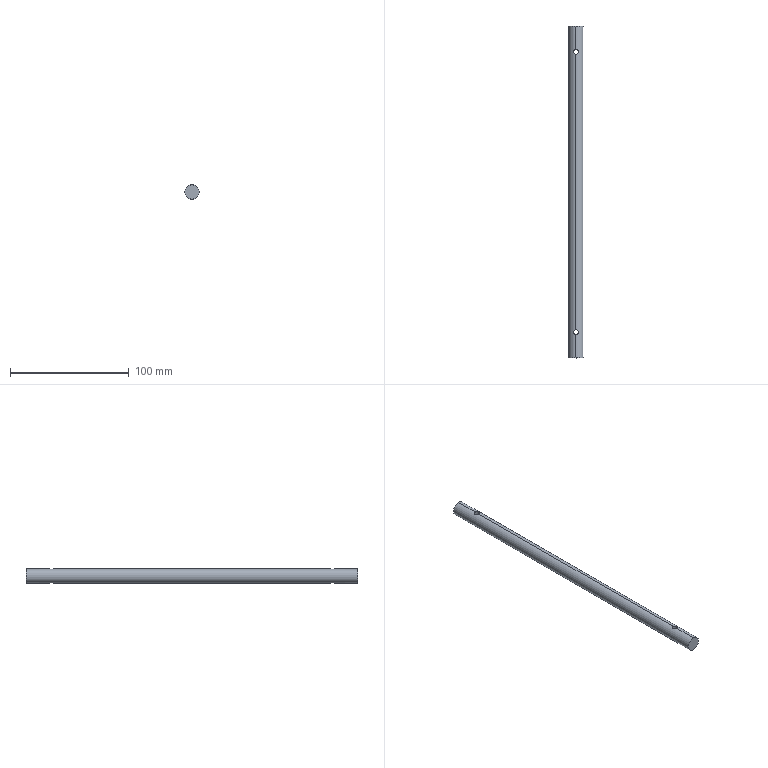Part | SolidWorks | features Extrusion 1, ICE 1, MirrorPattern 1 | 1 solid | 8 faces | box 12 x 280 x 12 mm | volume 31370 mm3 | cylinder 6 | plane 2 | commonest cylinder face diameters 4 x4 12 x2
STEP:
#1=CARTESIAN_POINT('',(0.,116.208,-6.));
#2=VERTEX_POINT('',#1);
#3=CARTESIAN_POINT('',(-2.,118.208,-5.657));
#4=VERTEX_POINT('',#3);
#5=CARTESIAN_POINT('',(0.,116.208,-6.));
#6=CARTESIAN_POINT('',(-0.2623,116.208,-6.));
#7=CARTESIAN_POINT('',(-0.5271,116.261,-5.982));
#8=CARTESIAN_POINT('',(-0.889,116.412,-5.935));
#9=CARTESIAN_POINT('',(-1.006,116.475,-5.916));
#10=CARTESIAN_POINT('',(-1.222,116.619,-5.875));
#11=CARTESIAN_POINT('',(-1.322,116.702,-5.853));
#12=CARTESIAN_POINT('',(-1.599,116.979,-5.786));
#13=CARTESIAN_POINT('',(-1.745,117.197,-5.741));
#14=CARTESIAN_POINT('',(-1.897,117.561,-5.692));
#15=CARTESIAN_POINT('',(-1.935,117.686,-5.679));
#16=CARTESIAN_POINT('',(-1.987,117.943,-5.662));
#17=CARTESIAN_POINT('',(-2.,118.076,-5.657));
#18=CARTESIAN_POINT('',(-2.,118.208,-5.657));
#19=B_SPLINE_CURVE_WITH_KNOTS('',3,(#5,#6,#7,#8,#9,#10,#11,#12,#13,#14,#15,#16,#17,#18),.UNSPECIFIED.,.F.,.F.,(4,2,2,2,2,2,4),(0.006298,0.007085,0.007479,0.007872,0.008659,0.009053,0.009446),.UNSPECIFIED.);
#20=EDGE_CURVE('',#2,#4,#19,.T.);
#21=ORIENTED_EDGE('',*,*,#20,.T.);
#22=CARTESIAN_POINT('',(-2.,118.208,5.657));
#23=VERTEX_POINT('',#22);
#24=CARTESIAN_POINT('',(-2.,118.208,-49.));
#25=DIRECTION('',(0.,0.,1.));
#26=VECTOR('',#25,1000.);
#27=LINE('',#24,#26);
#28=EDGE_CURVE('',#4,#23,#27,.T.);
#29=ORIENTED_EDGE('',*,*,#28,.T.);
#30=CARTESIAN_POINT('',(0.,116.208,6.));
#31=VERTEX_POINT('',#30);
#32=CARTESIAN_POINT('',(-2.,118.208,5.657));
#33=CARTESIAN_POINT('',(-2.,117.946,5.657));
#34=CARTESIAN_POINT('',(-1.947,117.681,5.676));
#35=CARTESIAN_POINT('',(-1.796,117.319,5.725));
#36=CARTESIAN_POINT('',(-1.734,117.202,5.745));
#37=CARTESIAN_POINT('',(-1.589,116.987,5.786));
#38=CARTESIAN_POINT('',(-1.507,116.886,5.809));
#39=CARTESIAN_POINT('',(-1.23,116.609,5.876));
#40=CARTESIAN_POINT('',(-1.012,116.463,5.919));
#41=CARTESIAN_POINT('',(-0.6469,116.311,5.966));
#42=CARTESIAN_POINT('',(-0.5219,116.273,5.979));
#43=CARTESIAN_POINT('',(-0.2652,116.221,5.996));
#44=CARTESIAN_POINT('',(-0.1318,116.208,6.));
#45=CARTESIAN_POINT('',(0.,116.208,6.));
#46=B_SPLINE_CURVE_WITH_KNOTS('',3,(#32,#33,#34,#35,#36,#37,#38,#39,#40,#41,#42,#43,#44,#45),.UNSPECIFIED.,.F.,.F.,(4,2,2,2,2,2,4),(0.006298,0.007085,0.007479,0.007872,0.008659,0.009053,0.009446),.UNSPECIFIED.);
#47=EDGE_CURVE('',#23,#31,#46,.T.);
#48=ORIENTED_EDGE('',*,*,#47,.T.);
#49=CARTESIAN_POINT('',(2.,118.208,5.657));
#50=VERTEX_POINT('',#49);
#51=CARTESIAN_POINT('',(0.,116.208,6.));
#52=CARTESIAN_POINT('',(0.1318,116.208,6.));
#53=CARTESIAN_POINT('',(0.2623,116.221,5.996));
#54=CARTESIAN_POINT('',(0.5209,116.273,5.979));
#55=CARTESIAN_POINT('',(0.6482,116.312,5.966));
#56=CARTESIAN_POINT('',(1.01,116.462,5.919));
#57=CARTESIAN_POINT('',(1.231,116.611,5.875));
#58=CARTESIAN_POINT('',(1.506,116.886,5.809));
#59=CARTESIAN_POINT('',(1.59,116.988,5.786));
#60=CARTESIAN_POINT('',(1.734,117.204,5.744));
#61=CARTESIAN_POINT('',(1.796,117.318,5.725));
#62=CARTESIAN_POINT('',(1.897,117.56,5.693));
#63=CARTESIAN_POINT('',(1.935,117.687,5.679));
#64=CARTESIAN_POINT('',(1.987,117.944,5.662));
#65=CARTESIAN_POINT('',(2.,118.075,5.657));
#66=CARTESIAN_POINT('',(2.,118.208,5.657));
#67=B_SPLINE_CURVE_WITH_KNOTS('',3,(#51,#52,#53,#54,#55,#56,#57,#58,#59,#60,#61,#62,#63,#64,#65,#66),.UNSPECIFIED.,.F.,.F.,(4,2,2,2,2,2,2,4),(0.009446,0.00984,0.01023,0.01102,0.01141,0.01181,0.0122,0.01259),.UNSPECIFIED.);
#68=EDGE_CURVE('',#31,#50,#67,.T.);
#69=ORIENTED_EDGE('',*,*,#68,.T.);
#70=CARTESIAN_POINT('',(2.,118.208,-5.657));
#71=VERTEX_POINT('',#70);
#72=CARTESIAN_POINT('',(2.,118.208,-49.));
#73=DIRECTION('',(0.,0.,1.));
#74=VECTOR('',#73,1000.);
#75=LINE('',#72,#74);
#76=EDGE_CURVE('',#71,#50,#75,.T.);
#77=ORIENTED_EDGE('',*,*,#76,.F.);
#78=CARTESIAN_POINT('',(2.,118.208,-5.657));
#79=CARTESIAN_POINT('',(2.,118.077,-5.657));
#80=CARTESIAN_POINT('',(1.987,117.943,-5.662));
#81=CARTESIAN_POINT('',(1.935,117.686,-5.679));
#82=CARTESIAN_POINT('',(1.897,117.561,-5.693));
#83=CARTESIAN_POINT('',(1.796,117.317,-5.725));
#84=CARTESIAN_POINT('',(1.734,117.202,-5.745));
#85=CARTESIAN_POINT('',(1.589,116.987,-5.786));
#86=CARTESIAN_POINT('',(1.505,116.885,-5.809));
#87=CARTESIAN_POINT('',(1.321,116.701,-5.853));
#88=CARTESIAN_POINT('',(1.221,116.619,-5.875));
#89=CARTESIAN_POINT('',(1.005,116.474,-5.916));
#90=CARTESIAN_POINT('',(0.8882,116.411,-5.935));
#91=CARTESIAN_POINT('',(0.6474,116.311,-5.966));
#92=CARTESIAN_POINT('',(0.5226,116.273,-5.979));
#93=CARTESIAN_POINT('',(0.2637,116.221,-5.996));
#94=CARTESIAN_POINT('',(0.1311,116.208,-6.));
#95=CARTESIAN_POINT('',(0.,116.208,-6.));
#96=B_SPLINE_CURVE_WITH_KNOTS('',3,(#78,#79,#80,#81,#82,#83,#84,#85,#86,#87,#88,#89,#90,#91,#92,#93,#94,#95),.UNSPECIFIED.,.F.,.F.,(4,2,2,2,2,2,2,2,4),(0.00315,0.003544,0.003937,0.004331,0.004724,0.005118,0.005511,0.005905,0.006298),.UNSPECIFIED.);
#97=EDGE_CURVE('',#71,#2,#96,.T.);
#98=ORIENTED_EDGE('',*,*,#97,.T.);
#99=EDGE_LOOP('',(#21,#29,#48,#69,#77,#98));
#100=FACE_OUTER_BOUND('',#99,.T.);
#101=CARTESIAN_POINT('',(0.,118.208,-49.));
#102=DIRECTION('',(0.,0.,1.));
#103=DIRECTION('',(1.,0.,0.));
#104=AXIS2_PLACEMENT_3D('',#101,#102,#103);
#105=CYLINDRICAL_SURFACE('',#104,2.);
#106=ADVANCED_FACE('',(#100),#105,.F.);
#107=CARTESIAN_POINT('',(-2.,-118.208,-5.657));
#108=VERTEX_POINT('',#107);
#109=CARTESIAN_POINT('',(0.,-120.208,-6.));
#110=VERTEX_POINT('',#109);
#111=CARTESIAN_POINT('',(-2.,-118.208,-5.657));
#112=CARTESIAN_POINT('',(-2.,-118.34,-5.657));
#113=CARTESIAN_POINT('',(-1.987,-118.473,-5.662));
#114=CARTESIAN_POINT('',(-1.935,-118.73,-5.679));
#115=CARTESIAN_POINT('',(-1.897,-118.855,-5.693));
#116=CARTESIAN_POINT('',(-1.796,-119.099,-5.725));
#117=CARTESIAN_POINT('',(-1.734,-119.214,-5.745));
#118=CARTESIAN_POINT('',(-1.589,-119.429,-5.786));
#119=CARTESIAN_POINT('',(-1.505,-119.531,-5.809));
#120=CARTESIAN_POINT('',(-1.321,-119.715,-5.853));
#121=CARTESIAN_POINT('',(-1.221,-119.797,-5.875));
#122=CARTESIAN_POINT('',(-1.005,-119.942,-5.916));
#123=CARTESIAN_POINT('',(-0.8882,-120.005,-5.935));
#124=CARTESIAN_POINT('',(-0.6474,-120.105,-5.966));
#125=CARTESIAN_POINT('',(-0.5226,-120.143,-5.979));
#126=CARTESIAN_POINT('',(-0.2637,-120.195,-5.996));
#127=CARTESIAN_POINT('',(-0.1311,-120.208,-6.));
#128=CARTESIAN_POINT('',(0.,-120.208,-6.));
#129=B_SPLINE_CURVE_WITH_KNOTS('',3,(#111,#112,#113,#114,#115,#116,#117,#118,#119,#120,#121,#122,#123,#124,#125,#126,#127,#128),.UNSPECIFIED.,.F.,.F.,(4,2,2,2,2,2,2,2,4),(0.00315,0.003544,0.003937,0.004331,0.004724,0.005118,0.005511,0.005905,0.006298),.UNSPECIFIED.);
#130=EDGE_CURVE('',#108,#110,#129,.T.);
#131=ORIENTED_EDGE('',*,*,#130,.F.);
#132=CARTESIAN_POINT('',(-2.,-118.208,5.657));
#133=VERTEX_POINT('',#132);
#134=CARTESIAN_POINT('',(-2.,-118.208,-49.));
#135=DIRECTION('',(0.,0.,1.));
#136=VECTOR('',#135,1000.);
#137=LINE('',#134,#136);
#138=EDGE_CURVE('',#108,#133,#137,.T.);
#139=ORIENTED_EDGE('',*,*,#138,.T.);
#140=CARTESIAN_POINT('',(0.,-120.208,6.));
#141=VERTEX_POINT('',#140);
#142=CARTESIAN_POINT('',(0.,-120.208,6.));
#143=CARTESIAN_POINT('',(-0.1315,-120.208,6.));
#144=CARTESIAN_POINT('',(-0.2651,-120.195,5.996));
#145=CARTESIAN_POINT('',(-0.5223,-120.143,5.979));
#146=CARTESIAN_POINT('',(-0.6475,-120.105,5.966));
#147=CARTESIAN_POINT('',(-0.8909,-120.004,5.935));
#148=CARTESIAN_POINT('',(-1.006,-119.941,5.916));
#149=CARTESIAN_POINT('',(-1.222,-119.797,5.875));
#150=CARTESIAN_POINT('',(-1.324,-119.713,5.853));
#151=CARTESIAN_POINT('',(-1.507,-119.529,5.808));
#152=CARTESIAN_POINT('',(-1.589,-119.429,5.786));
#153=CARTESIAN_POINT('',(-1.734,-119.213,5.744));
#154=CARTESIAN_POINT('',(-1.797,-119.096,5.725));
#155=CARTESIAN_POINT('',(-1.897,-118.855,5.693));
#156=CARTESIAN_POINT('',(-1.935,-118.731,5.679));
#157=CARTESIAN_POINT('',(-1.987,-118.472,5.662));
#158=CARTESIAN_POINT('',(-2.,-118.339,5.657));
#159=CARTESIAN_POINT('',(-2.,-118.208,5.657));
#160=B_SPLINE_CURVE_WITH_KNOTS('',3,(#142,#143,#144,#145,#146,#147,#148,#149,#150,#151,#152,#153,#154,#155,#156,#157,#158,#159),.UNSPECIFIED.,.F.,.F.,(4,2,2,2,2,2,2,2,4),(0.00315,0.003544,0.003937,0.004331,0.004724,0.005118,0.005511,0.005905,0.006298),.UNSPECIFIED.);
#161=EDGE_CURVE('',#141,#133,#160,.T.);
#162=ORIENTED_EDGE('',*,*,#161,.F.);
#163=CARTESIAN_POINT('',(2.,-118.208,5.657));
#164=VERTEX_POINT('',#163);
#165=CARTESIAN_POINT('',(2.,-118.208,5.657));
#166=CARTESIAN_POINT('',(2.,-118.341,5.657));
#167=CARTESIAN_POINT('',(1.987,-118.472,5.662));
#168=CARTESIAN_POINT('',(1.935,-118.729,5.679));
#169=CARTESIAN_POINT('',(1.896,-118.857,5.693));
#170=CARTESIAN_POINT('',(1.796,-119.098,5.725));
#171=CARTESIAN_POINT('',(1.734,-119.213,5.744));
#172=CARTESIAN_POINT('',(1.589,-119.43,5.786));
#173=CARTESIAN_POINT('',(1.505,-119.531,5.809));
#174=CARTESIAN_POINT('',(1.23,-119.806,5.876));
#175=CARTESIAN_POINT('',(1.009,-119.955,5.92));
#176=CARTESIAN_POINT('',(0.648,-120.105,5.966));
#177=CARTESIAN_POINT('',(0.5209,-120.144,5.979));
#178=CARTESIAN_POINT('',(0.2621,-120.195,5.996));
#179=CARTESIAN_POINT('',(0.1316,-120.208,6.));
#180=CARTESIAN_POINT('',(0.,-120.208,6.));
#181=B_SPLINE_CURVE_WITH_KNOTS('',3,(#165,#166,#167,#168,#169,#170,#171,#172,#173,#174,#175,#176,#177,#178,#179,#180),.UNSPECIFIED.,.F.,.F.,(4,2,2,2,2,2,2,4),(0.,0.0003937,0.0007875,0.001181,0.001575,0.002362,0.002756,0.00315),.UNSPECIFIED.);
#182=EDGE_CURVE('',#164,#141,#181,.T.);
#183=ORIENTED_EDGE('',*,*,#182,.F.);
#184=CARTESIAN_POINT('',(2.,-118.208,-5.657));
#185=VERTEX_POINT('',#184);
#186=CARTESIAN_POINT('',(2.,-118.208,-49.));
#187=DIRECTION('',(0.,0.,1.));
#188=VECTOR('',#187,1000.);
#189=LINE('',#186,#188);
#190=EDGE_CURVE('',#185,#164,#189,.T.);
#191=ORIENTED_EDGE('',*,*,#190,.F.);
#192=CARTESIAN_POINT('',(0.,-120.208,-6.));
#193=CARTESIAN_POINT('',(0.2623,-120.208,-6.));
#194=CARTESIAN_POINT('',(0.5271,-120.155,-5.982));
#195=CARTESIAN_POINT('',(0.889,-120.004,-5.935));
#196=CARTESIAN_POINT('',(1.006,-119.942,-5.916));
#197=CARTESIAN_POINT('',(1.222,-119.797,-5.875));
#198=CARTESIAN_POINT('',(1.322,-119.714,-5.853));
#199=CARTESIAN_POINT('',(1.599,-119.437,-5.786));
#200=CARTESIAN_POINT('',(1.745,-119.219,-5.741));
#201=CARTESIAN_POINT('',(1.897,-118.855,-5.692));
#202=CARTESIAN_POINT('',(1.935,-118.73,-5.679));
#203=CARTESIAN_POINT('',(1.987,-118.473,-5.662));
#204=CARTESIAN_POINT('',(2.,-118.34,-5.657));
#205=CARTESIAN_POINT('',(2.,-118.208,-5.657));
#206=B_SPLINE_CURVE_WITH_KNOTS('',3,(#192,#193,#194,#195,#196,#197,#198,#199,#200,#201,#202,#203,#204,#205),.UNSPECIFIED.,.F.,.F.,(4,2,2,2,2,2,4),(0.006298,0.007085,0.007479,0.007872,0.008659,0.009053,0.009446),.UNSPECIFIED.);
#207=EDGE_CURVE('',#110,#185,#206,.T.);
#208=ORIENTED_EDGE('',*,*,#207,.F.);
#209=EDGE_LOOP('',(#131,#139,#162,#183,#191,#208));
#210=FACE_OUTER_BOUND('',#209,.T.);
#211=CARTESIAN_POINT('',(0.,-118.208,-49.));
#212=DIRECTION('',(0.,0.,1.));
#213=DIRECTION('',(1.,0.,0.));
#214=AXIS2_PLACEMENT_3D('',#211,#212,#213);
#215=CYLINDRICAL_SURFACE('',#214,2.);
#216=ADVANCED_FACE('',(#210),#215,.F.);
#217=CARTESIAN_POINT('',(0.,140.,6.));
#218=VERTEX_POINT('',#217);
#219=CARTESIAN_POINT('',(0.,140.,-6.));
#220=VERTEX_POINT('',#219);
#221=CARTESIAN_POINT('',(0.,140.,0.));
#222=DIRECTION('',(0.,1.,0.));
#223=DIRECTION('',(0.,0.,1.));
#224=AXIS2_PLACEMENT_3D('',#221,#222,#223);
#225=CIRCLE('',#224,6.);
#226=EDGE_CURVE('',#218,#220,#225,.T.);
#227=ORIENTED_EDGE('',*,*,#226,.F.);
#228=CARTESIAN_POINT('',(0.,120.208,6.));
#229=VERTEX_POINT('',#228);
#230=CARTESIAN_POINT('',(0.,140.,6.));
#231=DIRECTION('',(0.,-1.,0.));
#232=VECTOR('',#231,1000.);
#233=LINE('',#230,#232);
#234=EDGE_CURVE('',#218,#229,#233,.T.);
#235=ORIENTED_EDGE('',*,*,#234,.T.);
#236=CARTESIAN_POINT('',(2.,118.208,5.657));
#237=CARTESIAN_POINT('',(2.,118.341,5.657));
#238=CARTESIAN_POINT('',(1.987,118.472,5.662));
#239=CARTESIAN_POINT('',(1.935,118.729,5.679));
#240=CARTESIAN_POINT('',(1.896,118.857,5.693));
#241=CARTESIAN_POINT('',(1.796,119.098,5.725));
#242=CARTESIAN_POINT('',(1.734,119.213,5.744));
#243=CARTESIAN_POINT('',(1.589,119.43,5.786));
#244=CARTESIAN_POINT('',(1.505,119.531,5.809));
#245=CARTESIAN_POINT('',(1.23,119.806,5.876));
#246=CARTESIAN_POINT('',(1.009,119.955,5.92));
#247=CARTESIAN_POINT('',(0.648,120.105,5.966));
#248=CARTESIAN_POINT('',(0.5209,120.144,5.979));
#249=CARTESIAN_POINT('',(0.2621,120.195,5.996));
#250=CARTESIAN_POINT('',(0.1316,120.208,6.));
#251=CARTESIAN_POINT('',(0.,120.208,6.));
#252=B_SPLINE_CURVE_WITH_KNOTS('',3,(#236,#237,#238,#239,#240,#241,#242,#243,#244,#245,#246,#247,#248,#249,#250,#251),.UNSPECIFIED.,.F.,.F.,(4,2,2,2,2,2,2,4),(0.,0.0003937,0.0007875,0.001181,0.001575,0.002362,0.002756,0.00315),.UNSPECIFIED.);
#253=EDGE_CURVE('',#50,#229,#252,.T.);
#254=ORIENTED_EDGE('',*,*,#253,.F.);
#255=ORIENTED_EDGE('',*,*,#68,.F.);
#256=CARTESIAN_POINT('',(0.,-116.208,6.));
#257=VERTEX_POINT('',#256);
#258=CARTESIAN_POINT('',(0.,140.,6.));
#259=DIRECTION('',(0.,-1.,0.));
#260=VECTOR('',#259,1000.);
#261=LINE('',#258,#260);
#262=EDGE_CURVE('',#31,#257,#261,.T.);
#263=ORIENTED_EDGE('',*,*,#262,.T.);
#264=CARTESIAN_POINT('',(0.,-116.208,6.));
#265=CARTESIAN_POINT('',(0.1318,-116.208,6.));
#266=CARTESIAN_POINT('',(0.2623,-116.221,5.996));
#267=CARTESIAN_POINT('',(0.5209,-116.273,5.979));
#268=CARTESIAN_POINT('',(0.6482,-116.312,5.966));
#269=CARTESIAN_POINT('',(1.01,-116.462,5.919));
#270=CARTESIAN_POINT('',(1.231,-116.611,5.875));
#271=CARTESIAN_POINT('',(1.506,-116.886,5.809));
#272=CARTESIAN_POINT('',(1.59,-116.988,5.786));
#273=CARTESIAN_POINT('',(1.734,-117.204,5.744));
#274=CARTESIAN_POINT('',(1.796,-117.318,5.725));
#275=CARTESIAN_POINT('',(1.897,-117.56,5.693));
#276=CARTESIAN_POINT('',(1.935,-117.687,5.679));
#277=CARTESIAN_POINT('',(1.987,-117.944,5.662));
#278=CARTESIAN_POINT('',(2.,-118.075,5.657));
#279=CARTESIAN_POINT('',(2.,-118.208,5.657));
#280=B_SPLINE_CURVE_WITH_KNOTS('',3,(#264,#265,#266,#267,#268,#269,#270,#271,#272,#273,#274,#275,#276,#277,#278,#279),.UNSPECIFIED.,.F.,.F.,(4,2,2,2,2,2,2,4),(0.009446,0.00984,0.01023,0.01102,0.01141,0.01181,0.0122,0.01259),.UNSPECIFIED.);
#281=EDGE_CURVE('',#257,#164,#280,.T.);
#282=ORIENTED_EDGE('',*,*,#281,.T.);
#283=ORIENTED_EDGE('',*,*,#182,.T.);
#284=CARTESIAN_POINT('',(0.,-140.,6.));
#285=VERTEX_POINT('',#284);
#286=CARTESIAN_POINT('',(0.,140.,6.));
#287=DIRECTION('',(0.,-1.,0.));
#288=VECTOR('',#287,1000.);
#289=LINE('',#286,#288);
#290=EDGE_CURVE('',#141,#285,#289,.T.);
#291=ORIENTED_EDGE('',*,*,#290,.T.);
#292=CARTESIAN_POINT('',(0.,-140.,-6.));
#293=VERTEX_POINT('',#292);
#294=CARTESIAN_POINT('',(0.,-140.,0.));
#295=DIRECTION('',(0.,1.,0.));
#296=DIRECTION('',(0.,0.,1.));
#297=AXIS2_PLACEMENT_3D('',#294,#295,#296);
#298=CIRCLE('',#297,6.);
#299=EDGE_CURVE('',#285,#293,#298,.T.);
#300=ORIENTED_EDGE('',*,*,#299,.T.);
#301=CARTESIAN_POINT('',(0.,140.,-6.));
#302=DIRECTION('',(0.,-1.,0.));
#303=VECTOR('',#302,1000.);
#304=LINE('',#301,#303);
#305=EDGE_CURVE('',#110,#293,#304,.T.);
#306=ORIENTED_EDGE('',*,*,#305,.F.);
#307=ORIENTED_EDGE('',*,*,#207,.T.);
#308=CARTESIAN_POINT('',(0.,-116.208,-6.));
#309=VERTEX_POINT('',#308);
#310=CARTESIAN_POINT('',(2.,-118.208,-5.657));
#311=CARTESIAN_POINT('',(2.,-118.076,-5.657));
#312=CARTESIAN_POINT('',(1.987,-117.946,-5.661));
#313=CARTESIAN_POINT('',(1.935,-117.687,-5.679));
#314=CARTESIAN_POINT('',(1.897,-117.56,-5.693));
#315=CARTESIAN_POINT('',(1.746,-117.199,-5.741));
#316=CARTESIAN_POINT('',(1.598,-116.978,-5.786));
#317=CARTESIAN_POINT('',(1.323,-116.702,-5.853));
#318=CARTESIAN_POINT('',(1.221,-116.619,-5.876));
#319=CARTESIAN_POINT('',(1.005,-116.474,-5.916));
#320=CARTESIAN_POINT('',(0.8903,-116.412,-5.935));
#321=CARTESIAN_POINT('',(0.6484,-116.312,-5.966));
#322=CARTESIAN_POINT('',(0.5209,-116.273,-5.979));
#323=CARTESIAN_POINT('',(0.264,-116.221,-5.996));
#324=CARTESIAN_POINT('',(0.1331,-116.208,-6.));
#325=CARTESIAN_POINT('',(0.,-116.208,-6.));
#326=B_SPLINE_CURVE_WITH_KNOTS('',3,(#310,#311,#312,#313,#314,#315,#316,#317,#318,#319,#320,#321,#322,#323,#324,#325),.UNSPECIFIED.,.F.,.F.,(4,2,2,2,2,2,2,4),(0.009446,0.00984,0.01023,0.01102,0.01141,0.01181,0.0122,0.0126),.UNSPECIFIED.);
#327=EDGE_CURVE('',#185,#309,#326,.T.);
#328=ORIENTED_EDGE('',*,*,#327,.T.);
#329=CARTESIAN_POINT('',(0.,140.,-6.));
#330=DIRECTION('',(0.,-1.,0.));
#331=VECTOR('',#330,1000.);
#332=LINE('',#329,#331);
#333=EDGE_CURVE('',#2,#309,#332,.T.);
#334=ORIENTED_EDGE('',*,*,#333,.F.);
#335=ORIENTED_EDGE('',*,*,#97,.F.);
#336=CARTESIAN_POINT('',(0.,120.208,-6.));
#337=VERTEX_POINT('',#336);
#338=CARTESIAN_POINT('',(0.,120.208,-6.));
#339=CARTESIAN_POINT('',(0.1332,120.208,-6.));
#340=CARTESIAN_POINT('',(0.264,120.195,-5.996));
#341=CARTESIAN_POINT('',(0.5211,120.143,-5.979));
#342=CARTESIAN_POINT('',(0.6487,120.104,-5.966));
#343=CARTESIAN_POINT('',(0.8906,120.004,-5.935));
#344=CARTESIAN_POINT('',(1.005,119.942,-5.916));
#345=CARTESIAN_POINT('',(1.222,119.797,-5.875));
#346=CARTESIAN_POINT('',(1.324,119.713,-5.853));
#347=CARTESIAN_POINT('',(1.598,119.438,-5.786));
#348=CARTESIAN_POINT('',(1.747,119.216,-5.741));
#349=CARTESIAN_POINT('',(1.897,118.856,-5.693));
#350=CARTESIAN_POINT('',(1.936,118.729,-5.679));
#351=CARTESIAN_POINT('',(1.987,118.47,-5.661));
#352=CARTESIAN_POINT('',(2.,118.34,-5.657));
#353=CARTESIAN_POINT('',(2.,118.208,-5.657));
#354=B_SPLINE_CURVE_WITH_KNOTS('',3,(#338,#339,#340,#341,#342,#343,#344,#345,#346,#347,#348,#349,#350,#351,#352,#353),.UNSPECIFIED.,.F.,.F.,(4,2,2,2,2,2,2,4),(0.,0.0003938,0.0007875,0.001181,0.001575,0.002363,0.002756,0.00315),.UNSPECIFIED.);
#355=EDGE_CURVE('',#337,#71,#354,.T.);
#356=ORIENTED_EDGE('',*,*,#355,.F.);
#357=CARTESIAN_POINT('',(0.,140.,-6.));
#358=DIRECTION('',(0.,-1.,0.));
#359=VECTOR('',#358,1000.);
#360=LINE('',#357,#359);
#361=EDGE_CURVE('',#220,#337,#360,.T.);
#362=ORIENTED_EDGE('',*,*,#361,.F.);
#363=EDGE_LOOP('',(#227,#235,#254,#255,#263,#282,#283,#291,#300,#306,#307,#328,#334,#335,#356,#362));
#364=FACE_OUTER_BOUND('',#363,.T.);
#365=CARTESIAN_POINT('',(0.,140.,0.));
#366=DIRECTION('',(0.,-1.,0.));
#367=DIRECTION('',(0.,0.,-1.));
#368=AXIS2_PLACEMENT_3D('',#365,#366,#367);
#369=CYLINDRICAL_SURFACE('',#368,6.);
#370=ADVANCED_FACE('',(#364),#369,.T.);
#371=ORIENTED_EDGE('',*,*,#234,.F.);
#372=CARTESIAN_POINT('',(0.,140.,0.));
#373=DIRECTION('',(0.,1.,0.));
#374=DIRECTION('',(0.,0.,1.));
#375=AXIS2_PLACEMENT_3D('',#372,#373,#374);
#376=CIRCLE('',#375,6.);
#377=EDGE_CURVE('',#220,#218,#376,.T.);
#378=ORIENTED_EDGE('',*,*,#377,.F.);
#379=ORIENTED_EDGE('',*,*,#361,.T.);
#380=CARTESIAN_POINT('',(-2.,118.208,-5.657));
#381=CARTESIAN_POINT('',(-2.,118.34,-5.657));
#382=CARTESIAN_POINT('',(-1.987,118.47,-5.661));
#383=CARTESIAN_POINT('',(-1.935,118.729,-5.679));
#384=CARTESIAN_POINT('',(-1.897,118.856,-5.693));
#385=CARTESIAN_POINT('',(-1.746,119.217,-5.741));
#386=CARTESIAN_POINT('',(-1.598,119.439,-5.786));
#387=CARTESIAN_POINT('',(-1.323,119.714,-5.853));
#388=CARTESIAN_POINT('',(-1.221,119.798,-5.876));
#389=CARTESIAN_POINT('',(-1.005,119.942,-5.916));
#390=CARTESIAN_POINT('',(-0.8903,120.004,-5.935));
#391=CARTESIAN_POINT('',(-0.6484,120.105,-5.966));
#392=CARTESIAN_POINT('',(-0.5209,120.143,-5.979));
#393=CARTESIAN_POINT('',(-0.264,120.195,-5.996));
#394=CARTESIAN_POINT('',(-0.1331,120.208,-6.));
#395=CARTESIAN_POINT('',(0.,120.208,-6.));
#396=B_SPLINE_CURVE_WITH_KNOTS('',3,(#380,#381,#382,#383,#384,#385,#386,#387,#388,#389,#390,#391,#392,#393,#394,#395),.UNSPECIFIED.,.F.,.F.,(4,2,2,2,2,2,2,4),(0.009446,0.00984,0.01023,0.01102,0.01141,0.01181,0.0122,0.0126),.UNSPECIFIED.);
#397=EDGE_CURVE('',#4,#337,#396,.T.);
#398=ORIENTED_EDGE('',*,*,#397,.F.);
#399=ORIENTED_EDGE('',*,*,#20,.F.);
#400=ORIENTED_EDGE('',*,*,#333,.T.);
#401=CARTESIAN_POINT('',(0.,-116.208,-6.));
#402=CARTESIAN_POINT('',(-0.1332,-116.208,-6.));
#403=CARTESIAN_POINT('',(-0.264,-116.221,-5.996));
#404=CARTESIAN_POINT('',(-0.5211,-116.273,-5.979));
#405=CARTESIAN_POINT('',(-0.6487,-116.312,-5.966));
#406=CARTESIAN_POINT('',(-0.8906,-116.412,-5.935));
#407=CARTESIAN_POINT('',(-1.005,-116.474,-5.916));
#408=CARTESIAN_POINT('',(-1.222,-116.619,-5.875));
#409=CARTESIAN_POINT('',(-1.324,-116.703,-5.853));
#410=CARTESIAN_POINT('',(-1.598,-116.978,-5.786));
#411=CARTESIAN_POINT('',(-1.747,-117.2,-5.741));
#412=CARTESIAN_POINT('',(-1.897,-117.56,-5.693));
#413=CARTESIAN_POINT('',(-1.936,-117.687,-5.679));
#414=CARTESIAN_POINT('',(-1.987,-117.946,-5.661));
#415=CARTESIAN_POINT('',(-2.,-118.076,-5.657));
#416=CARTESIAN_POINT('',(-2.,-118.208,-5.657));
#417=B_SPLINE_CURVE_WITH_KNOTS('',3,(#401,#402,#403,#404,#405,#406,#407,#408,#409,#410,#411,#412,#413,#414,#415,#416),.UNSPECIFIED.,.F.,.F.,(4,2,2,2,2,2,2,4),(0.,0.0003938,0.0007875,0.001181,0.001575,0.002363,0.002756,0.00315),.UNSPECIFIED.);
#418=EDGE_CURVE('',#309,#108,#417,.T.);
#419=ORIENTED_EDGE('',*,*,#418,.T.);
#420=ORIENTED_EDGE('',*,*,#130,.T.);
#421=ORIENTED_EDGE('',*,*,#305,.T.);
#422=CARTESIAN_POINT('',(0.,-140.,0.));
#423=DIRECTION('',(0.,1.,0.));
#424=DIRECTION('',(0.,0.,1.));
#425=AXIS2_PLACEMENT_3D('',#422,#423,#424);
#426=CIRCLE('',#425,6.);
#427=EDGE_CURVE('',#293,#285,#426,.T.);
#428=ORIENTED_EDGE('',*,*,#427,.T.);
#429=ORIENTED_EDGE('',*,*,#290,.F.);
#430=ORIENTED_EDGE('',*,*,#161,.T.);
#431=CARTESIAN_POINT('',(-2.,-118.208,5.657));
#432=CARTESIAN_POINT('',(-2.,-117.946,5.657));
#433=CARTESIAN_POINT('',(-1.947,-117.681,5.676));
#434=CARTESIAN_POINT('',(-1.796,-117.319,5.725));
#435=CARTESIAN_POINT('',(-1.734,-117.202,5.745));
#436=CARTESIAN_POINT('',(-1.589,-116.987,5.786));
#437=CARTESIAN_POINT('',(-1.507,-116.886,5.809));
#438=CARTESIAN_POINT('',(-1.23,-116.609,5.876));
#439=CARTESIAN_POINT('',(-1.012,-116.463,5.919));
#440=CARTESIAN_POINT('',(-0.6469,-116.311,5.966));
#441=CARTESIAN_POINT('',(-0.5219,-116.273,5.979));
#442=CARTESIAN_POINT('',(-0.2652,-116.221,5.996));
#443=CARTESIAN_POINT('',(-0.1318,-116.208,6.));
#444=CARTESIAN_POINT('',(0.,-116.208,6.));
#445=B_SPLINE_CURVE_WITH_KNOTS('',3,(#431,#432,#433,#434,#435,#436,#437,#438,#439,#440,#441,#442,#443,#444),.UNSPECIFIED.,.F.,.F.,(4,2,2,2,2,2,4),(0.006298,0.007085,0.007479,0.007872,0.008659,0.009053,0.009446),.UNSPECIFIED.);
#446=EDGE_CURVE('',#133,#257,#445,.T.);
#447=ORIENTED_EDGE('',*,*,#446,.T.);
#448=ORIENTED_EDGE('',*,*,#262,.F.);
#449=ORIENTED_EDGE('',*,*,#47,.F.);
#450=CARTESIAN_POINT('',(0.,120.208,6.));
#451=CARTESIAN_POINT('',(-0.1315,120.208,6.));
#452=CARTESIAN_POINT('',(-0.2651,120.195,5.996));
#453=CARTESIAN_POINT('',(-0.5223,120.143,5.979));
#454=CARTESIAN_POINT('',(-0.6475,120.105,5.966));
#455=CARTESIAN_POINT('',(-0.8909,120.004,5.935));
#456=CARTESIAN_POINT('',(-1.006,119.941,5.916));
#457=CARTESIAN_POINT('',(-1.222,119.797,5.875));
#458=CARTESIAN_POINT('',(-1.324,119.713,5.853));
#459=CARTESIAN_POINT('',(-1.507,119.529,5.808));
#460=CARTESIAN_POINT('',(-1.589,119.429,5.786));
#461=CARTESIAN_POINT('',(-1.734,119.213,5.744));
#462=CARTESIAN_POINT('',(-1.797,119.096,5.725));
#463=CARTESIAN_POINT('',(-1.897,118.855,5.693));
#464=CARTESIAN_POINT('',(-1.935,118.731,5.679));
#465=CARTESIAN_POINT('',(-1.987,118.472,5.662));
#466=CARTESIAN_POINT('',(-2.,118.339,5.657));
#467=CARTESIAN_POINT('',(-2.,118.208,5.657));
#468=B_SPLINE_CURVE_WITH_KNOTS('',3,(#450,#451,#452,#453,#454,#455,#456,#457,#458,#459,#460,#461,#462,#463,#464,#465,#466,#467),.UNSPECIFIED.,.F.,.F.,(4,2,2,2,2,2,2,2,4),(0.00315,0.003544,0.003937,0.004331,0.004724,0.005118,0.005511,0.005905,0.006298),.UNSPECIFIED.);
#469=EDGE_CURVE('',#229,#23,#468,.T.);
#470=ORIENTED_EDGE('',*,*,#469,.F.);
#471=EDGE_LOOP('',(#371,#378,#379,#398,#399,#400,#419,#420,#421,#428,#429,#430,#447,#448,#449,#470));
#472=FACE_OUTER_BOUND('',#471,.T.);
#473=CARTESIAN_POINT('',(0.,140.,0.));
#474=DIRECTION('',(0.,-1.,0.));
#475=DIRECTION('',(0.,0.,-1.));
#476=AXIS2_PLACEMENT_3D('',#473,#474,#475);
#477=CYLINDRICAL_SURFACE('',#476,6.);
#478=ADVANCED_FACE('',(#472),#477,.T.);
#479=ORIENTED_EDGE('',*,*,#377,.T.);
#480=ORIENTED_EDGE('',*,*,#226,.T.);
#481=EDGE_LOOP('',(#479,#480));
#482=FACE_OUTER_BOUND('',#481,.T.);
#483=CARTESIAN_POINT('',(0.,140.,0.));
#484=DIRECTION('',(0.,1.,0.));
#485=DIRECTION('',(0.,0.,1.));
#486=AXIS2_PLACEMENT_3D('',#483,#484,#485);
#487=PLANE('',#486);
#488=ADVANCED_FACE('',(#482),#487,.T.);
#489=ORIENTED_EDGE('',*,*,#427,.F.);
#490=ORIENTED_EDGE('',*,*,#299,.F.);
#491=EDGE_LOOP('',(#489,#490));
#492=FACE_OUTER_BOUND('',#491,.T.);
#493=CARTESIAN_POINT('',(0.,-140.,0.));
#494=DIRECTION('',(0.,1.,0.));
#495=DIRECTION('',(0.,0.,1.));
#496=AXIS2_PLACEMENT_3D('',#493,#494,#495);
#497=PLANE('',#496);
#498=ADVANCED_FACE('',(#492),#497,.F.);
#499=ORIENTED_EDGE('',*,*,#138,.F.);
#500=ORIENTED_EDGE('',*,*,#418,.F.);
#501=ORIENTED_EDGE('',*,*,#327,.F.);
#502=ORIENTED_EDGE('',*,*,#190,.T.);
#503=ORIENTED_EDGE('',*,*,#281,.F.);
#504=ORIENTED_EDGE('',*,*,#446,.F.);
#505=EDGE_LOOP('',(#499,#500,#501,#502,#503,#504));
#506=FACE_OUTER_BOUND('',#505,.T.);
#507=CARTESIAN_POINT('',(0.,-118.208,-49.));
#508=DIRECTION('',(0.,0.,1.));
#509=DIRECTION('',(1.,0.,0.));
#510=AXIS2_PLACEMENT_3D('',#507,#508,#509);
#511=CYLINDRICAL_SURFACE('',#510,2.);
#512=ADVANCED_FACE('',(#506),#511,.F.);
#513=ORIENTED_EDGE('',*,*,#28,.F.);
#514=ORIENTED_EDGE('',*,*,#397,.T.);
#515=ORIENTED_EDGE('',*,*,#355,.T.);
#516=ORIENTED_EDGE('',*,*,#76,.T.);
#517=ORIENTED_EDGE('',*,*,#253,.T.);
#518=ORIENTED_EDGE('',*,*,#469,.T.);
#519=EDGE_LOOP('',(#513,#514,#515,#516,#517,#518));
#520=FACE_OUTER_BOUND('',#519,.T.);
#521=CARTESIAN_POINT('',(0.,118.208,-49.));
#522=DIRECTION('',(0.,0.,1.));
#523=DIRECTION('',(1.,0.,0.));
#524=AXIS2_PLACEMENT_3D('',#521,#522,#523);
#525=CYLINDRICAL_SURFACE('',#524,2.);
#526=ADVANCED_FACE('',(#520),#525,.F.);
#527=CLOSED_SHELL('',(#106,#216,#370,#478,#488,#498,#512,#526));
#528=MANIFOLD_SOLID_BREP('',#527);
#529=CARTESIAN_POINT('',(0.,0.,0.));
#530=DIRECTION('',(0.,0.,1.));
#531=DIRECTION('',(1.,0.,0.));
#532=AXIS2_PLACEMENT_3D('',#529,#530,#531);
#533=(LENGTH_UNIT()NAMED_UNIT(*)SI_UNIT(.MILLI.,.METRE.));
#534=UNCERTAINTY_MEASURE_WITH_UNIT(LENGTH_MEASURE(0.00001),#533,'','');
#535=(NAMED_UNIT(*)PLANE_ANGLE_UNIT()SI_UNIT($,.RADIAN.));
#536=(NAMED_UNIT(*)SI_UNIT($,.STERADIAN.)SOLID_ANGLE_UNIT());
#537=(GEOMETRIC_REPRESENTATION_CONTEXT(3)GLOBAL_UNCERTAINTY_ASSIGNED_CONTEXT((#534))GLOBAL_UNIT_ASSIGNED_CONTEXT((#533,#535,#536))REPRESENTATION_CONTEXT('',''));
#538=ADVANCED_BREP_SHAPE_REPRESENTATION('',(#528,#532),#537);